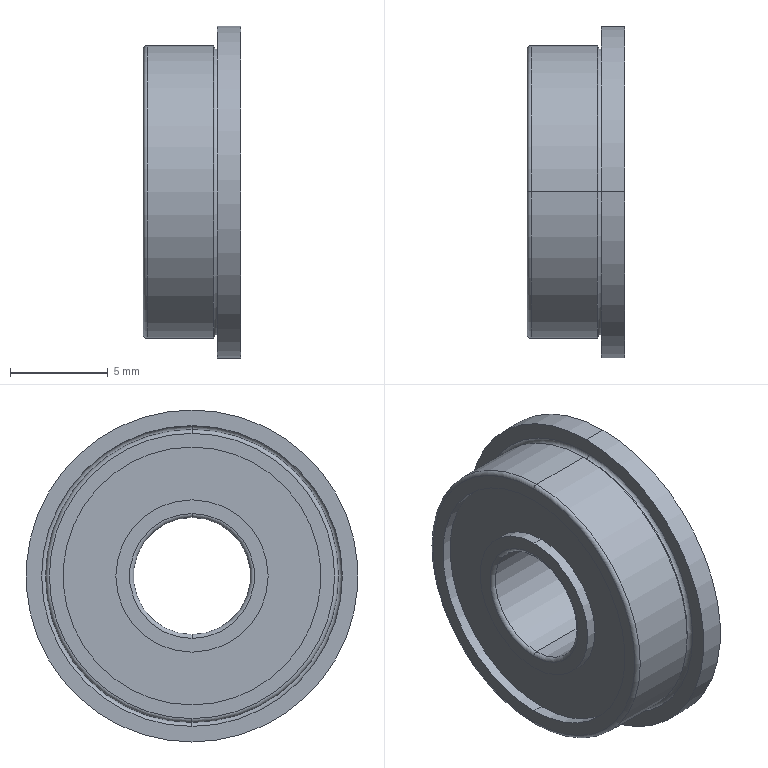Part | SolidWorks | features RefAxis 3, 3DProfileFeature 1, Revolution 1 | 1 solid | 31 faces | box 5 x 17 x 17 mm | volume 704.07 mm3 | cylinder 14 | torus 10 | plane 7 | commonest cylinder face diameters 7.8 x4 13.2 x4 6 x2 15 x2 17 x2
STEP:
#1=CARTESIAN_POINT('',(3.6,0.,7.5));
#2=VERTEX_POINT('',#1);
#3=CARTESIAN_POINT('',(3.8,0.,7.3));
#4=VERTEX_POINT('',#3);
#5=CARTESIAN_POINT('',(3.8,0.,7.5));
#6=DIRECTION('',(0.,-1.,0.));
#7=DIRECTION('',(0.,0.,-1.));
#8=AXIS2_PLACEMENT_3D('',#5,#6,#7);
#9=CIRCLE('',#8,0.2);
#10=EDGE_CURVE('',#2,#4,#9,.T.);
#11=ORIENTED_EDGE('',*,*,#10,.T.);
#12=CARTESIAN_POINT('',(3.8,0.,-7.3));
#13=VERTEX_POINT('',#12);
#14=CARTESIAN_POINT('',(3.8,0.,0.));
#15=DIRECTION('',(-1.,0.,0.));
#16=DIRECTION('',(0.,0.,1.));
#17=AXIS2_PLACEMENT_3D('',#14,#15,#16);
#18=CIRCLE('',#17,7.3);
#19=EDGE_CURVE('',#4,#13,#18,.T.);
#20=ORIENTED_EDGE('',*,*,#19,.T.);
#21=CARTESIAN_POINT('',(3.6,0.,-7.5));
#22=VERTEX_POINT('',#21);
#23=CARTESIAN_POINT('',(3.8,0.,-7.5));
#24=DIRECTION('',(0.,1.,0.));
#25=DIRECTION('',(0.,0.,1.));
#26=AXIS2_PLACEMENT_3D('',#23,#24,#25);
#27=CIRCLE('',#26,0.2);
#28=EDGE_CURVE('',#22,#13,#27,.T.);
#29=ORIENTED_EDGE('',*,*,#28,.F.);
#30=CARTESIAN_POINT('',(3.6,0.,0.));
#31=DIRECTION('',(-1.,0.,0.));
#32=DIRECTION('',(0.,0.,1.));
#33=AXIS2_PLACEMENT_3D('',#30,#31,#32);
#34=CIRCLE('',#33,7.5);
#35=EDGE_CURVE('',#2,#22,#34,.T.);
#36=ORIENTED_EDGE('',*,*,#35,.F.);
#37=EDGE_LOOP('',(#11,#20,#29,#36));
#38=FACE_OUTER_BOUND('',#37,.T.);
#39=CARTESIAN_POINT('',(3.8,0.,0.));
#40=DIRECTION('',(-1.,0.,0.));
#41=DIRECTION('',(0.,0.,1.));
#42=AXIS2_PLACEMENT_3D('',#39,#40,#41);
#43=TOROIDAL_SURFACE('',#42,7.5,0.2);
#44=ADVANCED_FACE('',(#38),#43,.F.);
#45=ORIENTED_EDGE('',*,*,#28,.T.);
#46=CARTESIAN_POINT('',(3.8,0.,0.));
#47=DIRECTION('',(-1.,0.,0.));
#48=DIRECTION('',(0.,0.,1.));
#49=AXIS2_PLACEMENT_3D('',#46,#47,#48);
#50=CIRCLE('',#49,7.3);
#51=EDGE_CURVE('',#13,#4,#50,.T.);
#52=ORIENTED_EDGE('',*,*,#51,.T.);
#53=ORIENTED_EDGE('',*,*,#10,.F.);
#54=CARTESIAN_POINT('',(3.6,0.,0.));
#55=DIRECTION('',(-1.,0.,0.));
#56=DIRECTION('',(0.,0.,1.));
#57=AXIS2_PLACEMENT_3D('',#54,#55,#56);
#58=CIRCLE('',#57,7.5);
#59=EDGE_CURVE('',#22,#2,#58,.T.);
#60=ORIENTED_EDGE('',*,*,#59,.F.);
#61=EDGE_LOOP('',(#45,#52,#53,#60));
#62=FACE_OUTER_BOUND('',#61,.T.);
#63=CARTESIAN_POINT('',(3.8,0.,0.));
#64=DIRECTION('',(-1.,0.,0.));
#65=DIRECTION('',(0.,0.,1.));
#66=AXIS2_PLACEMENT_3D('',#63,#64,#65);
#67=TOROIDAL_SURFACE('',#66,7.5,0.2);
#68=ADVANCED_FACE('',(#62),#67,.F.);
#69=ORIENTED_EDGE('',*,*,#35,.T.);
#70=CARTESIAN_POINT('',(0.2,0.,-7.5));
#71=VERTEX_POINT('',#70);
#72=CARTESIAN_POINT('',(15.,0.,-7.5));
#73=DIRECTION('',(-1.,0.,0.));
#74=VECTOR('',#73,1000.);
#75=LINE('',#72,#74);
#76=EDGE_CURVE('',#22,#71,#75,.T.);
#77=ORIENTED_EDGE('',*,*,#76,.T.);
#78=CARTESIAN_POINT('',(0.2,0.,7.5));
#79=VERTEX_POINT('',#78);
#80=CARTESIAN_POINT('',(0.2,0.,0.));
#81=DIRECTION('',(-1.,0.,0.));
#82=DIRECTION('',(0.,0.,1.));
#83=AXIS2_PLACEMENT_3D('',#80,#81,#82);
#84=CIRCLE('',#83,7.5);
#85=EDGE_CURVE('',#79,#71,#84,.T.);
#86=ORIENTED_EDGE('',*,*,#85,.F.);
#87=CARTESIAN_POINT('',(15.,0.,7.5));
#88=DIRECTION('',(-1.,0.,0.));
#89=VECTOR('',#88,1000.);
#90=LINE('',#87,#89);
#91=EDGE_CURVE('',#2,#79,#90,.T.);
#92=ORIENTED_EDGE('',*,*,#91,.F.);
#93=EDGE_LOOP('',(#69,#77,#86,#92));
#94=FACE_OUTER_BOUND('',#93,.T.);
#95=CARTESIAN_POINT('',(15.,0.,0.));
#96=DIRECTION('',(-1.,0.,0.));
#97=DIRECTION('',(0.,0.,1.));
#98=AXIS2_PLACEMENT_3D('',#95,#96,#97);
#99=CYLINDRICAL_SURFACE('',#98,7.5);
#100=ADVANCED_FACE('',(#94),#99,.T.);
#101=ORIENTED_EDGE('',*,*,#51,.F.);
#102=CARTESIAN_POINT('',(3.8,0.,-7.7));
#103=VERTEX_POINT('',#102);
#104=CARTESIAN_POINT('',(3.8,0.,-7.5));
#105=DIRECTION('',(0.,1.,0.));
#106=DIRECTION('',(0.,0.,1.));
#107=AXIS2_PLACEMENT_3D('',#104,#105,#106);
#108=CIRCLE('',#107,0.2);
#109=EDGE_CURVE('',#13,#103,#108,.T.);
#110=ORIENTED_EDGE('',*,*,#109,.T.);
#111=CARTESIAN_POINT('',(3.8,0.,7.7));
#112=VERTEX_POINT('',#111);
#113=CARTESIAN_POINT('',(3.8,0.,0.));
#114=DIRECTION('',(-1.,0.,0.));
#115=DIRECTION('',(0.,0.,1.));
#116=AXIS2_PLACEMENT_3D('',#113,#114,#115);
#117=CIRCLE('',#116,7.7);
#118=EDGE_CURVE('',#103,#112,#117,.T.);
#119=ORIENTED_EDGE('',*,*,#118,.T.);
#120=CARTESIAN_POINT('',(3.8,0.,7.5));
#121=DIRECTION('',(0.,-1.,0.));
#122=DIRECTION('',(0.,0.,-1.));
#123=AXIS2_PLACEMENT_3D('',#120,#121,#122);
#124=CIRCLE('',#123,0.2);
#125=EDGE_CURVE('',#4,#112,#124,.T.);
#126=ORIENTED_EDGE('',*,*,#125,.F.);
#127=EDGE_LOOP('',(#101,#110,#119,#126));
#128=FACE_OUTER_BOUND('',#127,.T.);
#129=CARTESIAN_POINT('',(3.8,0.,0.));
#130=DIRECTION('',(-1.,0.,0.));
#131=DIRECTION('',(0.,0.,1.));
#132=AXIS2_PLACEMENT_3D('',#129,#130,#131);
#133=TOROIDAL_SURFACE('',#132,7.5,0.2);
#134=ADVANCED_FACE('',(#128),#133,.F.);
#135=CARTESIAN_POINT('',(5.,0.,8.5));
#136=VERTEX_POINT('',#135);
#137=CARTESIAN_POINT('',(5.,0.,-8.5));
#138=VERTEX_POINT('',#137);
#139=CARTESIAN_POINT('',(5.,0.,0.));
#140=DIRECTION('',(-1.,0.,0.));
#141=DIRECTION('',(0.,0.,1.));
#142=AXIS2_PLACEMENT_3D('',#139,#140,#141);
#143=CIRCLE('',#142,8.5);
#144=EDGE_CURVE('',#136,#138,#143,.T.);
#145=ORIENTED_EDGE('',*,*,#144,.T.);
#146=CARTESIAN_POINT('',(3.8,0.,-8.5));
#147=VERTEX_POINT('',#146);
#148=CARTESIAN_POINT('',(15.,0.,-8.5));
#149=DIRECTION('',(-1.,0.,0.));
#150=VECTOR('',#149,1000.);
#151=LINE('',#148,#150);
#152=EDGE_CURVE('',#138,#147,#151,.T.);
#153=ORIENTED_EDGE('',*,*,#152,.T.);
#154=CARTESIAN_POINT('',(3.8,0.,8.5));
#155=VERTEX_POINT('',#154);
#156=CARTESIAN_POINT('',(3.8,0.,0.));
#157=DIRECTION('',(-1.,0.,0.));
#158=DIRECTION('',(0.,0.,1.));
#159=AXIS2_PLACEMENT_3D('',#156,#157,#158);
#160=CIRCLE('',#159,8.5);
#161=EDGE_CURVE('',#155,#147,#160,.T.);
#162=ORIENTED_EDGE('',*,*,#161,.F.);
#163=CARTESIAN_POINT('',(15.,0.,8.5));
#164=DIRECTION('',(-1.,0.,0.));
#165=VECTOR('',#164,1000.);
#166=LINE('',#163,#165);
#167=EDGE_CURVE('',#136,#155,#166,.T.);
#168=ORIENTED_EDGE('',*,*,#167,.F.);
#169=EDGE_LOOP('',(#145,#153,#162,#168));
#170=FACE_OUTER_BOUND('',#169,.T.);
#171=CARTESIAN_POINT('',(15.,0.,0.));
#172=DIRECTION('',(-1.,0.,0.));
#173=DIRECTION('',(0.,0.,1.));
#174=AXIS2_PLACEMENT_3D('',#171,#172,#173);
#175=CYLINDRICAL_SURFACE('',#174,8.5);
#176=ADVANCED_FACE('',(#170),#175,.T.);
#177=CARTESIAN_POINT('',(5.,0.,-6.6));
#178=VERTEX_POINT('',#177);
#179=CARTESIAN_POINT('',(5.,0.,6.6));
#180=VERTEX_POINT('',#179);
#181=CARTESIAN_POINT('',(5.,0.,0.));
#182=DIRECTION('',(-1.,0.,0.));
#183=DIRECTION('',(0.,0.,1.));
#184=AXIS2_PLACEMENT_3D('',#181,#182,#183);
#185=CIRCLE('',#184,6.6);
#186=EDGE_CURVE('',#178,#180,#185,.T.);
#187=ORIENTED_EDGE('',*,*,#186,.F.);
#188=CARTESIAN_POINT('',(4.476,0.,-6.6));
#189=VERTEX_POINT('',#188);
#190=CARTESIAN_POINT('',(15.,0.,-6.6));
#191=DIRECTION('',(-1.,0.,0.));
#192=VECTOR('',#191,1000.);
#193=LINE('',#190,#192);
#194=EDGE_CURVE('',#178,#189,#193,.T.);
#195=ORIENTED_EDGE('',*,*,#194,.T.);
#196=CARTESIAN_POINT('',(4.476,0.,6.6));
#197=VERTEX_POINT('',#196);
#198=CARTESIAN_POINT('',(4.476,0.,0.));
#199=DIRECTION('',(-1.,0.,0.));
#200=DIRECTION('',(0.,0.,1.));
#201=AXIS2_PLACEMENT_3D('',#198,#199,#200);
#202=CIRCLE('',#201,6.6);
#203=EDGE_CURVE('',#189,#197,#202,.T.);
#204=ORIENTED_EDGE('',*,*,#203,.T.);
#205=CARTESIAN_POINT('',(15.,0.,6.6));
#206=DIRECTION('',(-1.,0.,0.));
#207=VECTOR('',#206,1000.);
#208=LINE('',#205,#207);
#209=EDGE_CURVE('',#180,#197,#208,.T.);
#210=ORIENTED_EDGE('',*,*,#209,.F.);
#211=EDGE_LOOP('',(#187,#195,#204,#210));
#212=FACE_OUTER_BOUND('',#211,.T.);
#213=CARTESIAN_POINT('',(15.,0.,0.));
#214=DIRECTION('',(-1.,0.,0.));
#215=DIRECTION('',(0.,0.,1.));
#216=AXIS2_PLACEMENT_3D('',#213,#214,#215);
#217=CYLINDRICAL_SURFACE('',#216,6.6);
#218=ADVANCED_FACE('',(#212),#217,.F.);
#219=CARTESIAN_POINT('',(5.,0.,3.9));
#220=VERTEX_POINT('',#219);
#221=CARTESIAN_POINT('',(5.,0.,-3.9));
#222=VERTEX_POINT('',#221);
#223=CARTESIAN_POINT('',(5.,0.,0.));
#224=DIRECTION('',(-1.,0.,0.));
#225=DIRECTION('',(0.,0.,1.));
#226=AXIS2_PLACEMENT_3D('',#223,#224,#225);
#227=CIRCLE('',#226,3.9);
#228=EDGE_CURVE('',#220,#222,#227,.T.);
#229=ORIENTED_EDGE('',*,*,#228,.T.);
#230=CARTESIAN_POINT('',(4.476,0.,-3.9));
#231=VERTEX_POINT('',#230);
#232=CARTESIAN_POINT('',(15.,0.,-3.9));
#233=DIRECTION('',(-1.,0.,0.));
#234=VECTOR('',#233,1000.);
#235=LINE('',#232,#234);
#236=EDGE_CURVE('',#222,#231,#235,.T.);
#237=ORIENTED_EDGE('',*,*,#236,.T.);
#238=CARTESIAN_POINT('',(4.476,0.,3.9));
#239=VERTEX_POINT('',#238);
#240=CARTESIAN_POINT('',(4.476,0.,0.));
#241=DIRECTION('',(-1.,0.,0.));
#242=DIRECTION('',(0.,0.,1.));
#243=AXIS2_PLACEMENT_3D('',#240,#241,#242);
#244=CIRCLE('',#243,3.9);
#245=EDGE_CURVE('',#239,#231,#244,.T.);
#246=ORIENTED_EDGE('',*,*,#245,.F.);
#247=CARTESIAN_POINT('',(15.,0.,3.9));
#248=DIRECTION('',(-1.,0.,0.));
#249=VECTOR('',#248,1000.);
#250=LINE('',#247,#249);
#251=EDGE_CURVE('',#220,#239,#250,.T.);
#252=ORIENTED_EDGE('',*,*,#251,.F.);
#253=EDGE_LOOP('',(#229,#237,#246,#252));
#254=FACE_OUTER_BOUND('',#253,.T.);
#255=CARTESIAN_POINT('',(15.,0.,0.));
#256=DIRECTION('',(-1.,0.,0.));
#257=DIRECTION('',(0.,0.,1.));
#258=AXIS2_PLACEMENT_3D('',#255,#256,#257);
#259=CYLINDRICAL_SURFACE('',#258,3.9);
#260=ADVANCED_FACE('',(#254),#259,.T.);
#261=CARTESIAN_POINT('',(4.8,0.,3.));
#262=VERTEX_POINT('',#261);
#263=CARTESIAN_POINT('',(4.8,0.,-3.));
#264=VERTEX_POINT('',#263);
#265=CARTESIAN_POINT('',(4.8,0.,0.));
#266=DIRECTION('',(-1.,0.,0.));
#267=DIRECTION('',(0.,0.,1.));
#268=AXIS2_PLACEMENT_3D('',#265,#266,#267);
#269=CIRCLE('',#268,3.);
#270=EDGE_CURVE('',#262,#264,#269,.T.);
#271=ORIENTED_EDGE('',*,*,#270,.T.);
#272=CARTESIAN_POINT('',(5.,0.,-3.2));
#273=VERTEX_POINT('',#272);
#274=CARTESIAN_POINT('',(4.8,0.,-3.2));
#275=DIRECTION('',(0.,1.,0.));
#276=DIRECTION('',(0.,0.,1.));
#277=AXIS2_PLACEMENT_3D('',#274,#275,#276);
#278=CIRCLE('',#277,0.2);
#279=EDGE_CURVE('',#264,#273,#278,.T.);
#280=ORIENTED_EDGE('',*,*,#279,.T.);
#281=CARTESIAN_POINT('',(5.,0.,3.2));
#282=VERTEX_POINT('',#281);
#283=CARTESIAN_POINT('',(5.,0.,0.));
#284=DIRECTION('',(-1.,0.,0.));
#285=DIRECTION('',(0.,0.,1.));
#286=AXIS2_PLACEMENT_3D('',#283,#284,#285);
#287=CIRCLE('',#286,3.2);
#288=EDGE_CURVE('',#282,#273,#287,.T.);
#289=ORIENTED_EDGE('',*,*,#288,.F.);
#290=CARTESIAN_POINT('',(4.8,0.,3.2));
#291=DIRECTION('',(0.,-1.,0.));
#292=DIRECTION('',(0.,0.,-1.));
#293=AXIS2_PLACEMENT_3D('',#290,#291,#292);
#294=CIRCLE('',#293,0.2);
#295=EDGE_CURVE('',#262,#282,#294,.T.);
#296=ORIENTED_EDGE('',*,*,#295,.F.);
#297=EDGE_LOOP('',(#271,#280,#289,#296));
#298=FACE_OUTER_BOUND('',#297,.T.);
#299=CARTESIAN_POINT('',(4.8,0.,0.));
#300=DIRECTION('',(-1.,0.,0.));
#301=DIRECTION('',(0.,0.,1.));
#302=AXIS2_PLACEMENT_3D('',#299,#300,#301);
#303=TOROIDAL_SURFACE('',#302,3.2,0.2);
#304=ADVANCED_FACE('',(#298),#303,.T.);
#305=CARTESIAN_POINT('',(4.8,0.,0.));
#306=DIRECTION('',(-1.,0.,0.));
#307=DIRECTION('',(0.,0.,1.));
#308=AXIS2_PLACEMENT_3D('',#305,#306,#307);
#309=CIRCLE('',#308,3.);
#310=EDGE_CURVE('',#264,#262,#309,.T.);
#311=ORIENTED_EDGE('',*,*,#310,.F.);
#312=CARTESIAN_POINT('',(0.2,0.,-3.));
#313=VERTEX_POINT('',#312);
#314=CARTESIAN_POINT('',(15.,0.,-3.));
#315=DIRECTION('',(-1.,0.,0.));
#316=VECTOR('',#315,1000.);
#317=LINE('',#314,#316);
#318=EDGE_CURVE('',#264,#313,#317,.T.);
#319=ORIENTED_EDGE('',*,*,#318,.T.);
#320=CARTESIAN_POINT('',(0.2,0.,3.));
#321=VERTEX_POINT('',#320);
#322=CARTESIAN_POINT('',(0.2,0.,0.));
#323=DIRECTION('',(-1.,0.,0.));
#324=DIRECTION('',(0.,0.,1.));
#325=AXIS2_PLACEMENT_3D('',#322,#323,#324);
#326=CIRCLE('',#325,3.);
#327=EDGE_CURVE('',#313,#321,#326,.T.);
#328=ORIENTED_EDGE('',*,*,#327,.T.);
#329=CARTESIAN_POINT('',(15.,0.,3.));
#330=DIRECTION('',(-1.,0.,0.));
#331=VECTOR('',#330,1000.);
#332=LINE('',#329,#331);
#333=EDGE_CURVE('',#262,#321,#332,.T.);
#334=ORIENTED_EDGE('',*,*,#333,.F.);
#335=EDGE_LOOP('',(#311,#319,#328,#334));
#336=FACE_OUTER_BOUND('',#335,.T.);
#337=CARTESIAN_POINT('',(15.,0.,0.));
#338=DIRECTION('',(-1.,0.,0.));
#339=DIRECTION('',(0.,0.,1.));
#340=AXIS2_PLACEMENT_3D('',#337,#338,#339);
#341=CYLINDRICAL_SURFACE('',#340,3.);
#342=ADVANCED_FACE('',(#336),#341,.F.);
#343=CARTESIAN_POINT('',(0.,0.,3.2));
#344=VERTEX_POINT('',#343);
#345=CARTESIAN_POINT('',(0.,0.,-3.2));
#346=VERTEX_POINT('',#345);
#347=CARTESIAN_POINT('',(0.,0.,0.));
#348=DIRECTION('',(-1.,0.,0.));
#349=DIRECTION('',(0.,0.,1.));
#350=AXIS2_PLACEMENT_3D('',#347,#348,#349);
#351=CIRCLE('',#350,3.2);
#352=EDGE_CURVE('',#344,#346,#351,.T.);
#353=ORIENTED_EDGE('',*,*,#352,.T.);
#354=CARTESIAN_POINT('',(0.2,0.,-3.2));
#355=DIRECTION('',(0.,1.,0.));
#356=DIRECTION('',(0.,0.,1.));
#357=AXIS2_PLACEMENT_3D('',#354,#355,#356);
#358=CIRCLE('',#357,0.2);
#359=EDGE_CURVE('',#346,#313,#358,.T.);
#360=ORIENTED_EDGE('',*,*,#359,.T.);
#361=CARTESIAN_POINT('',(0.2,0.,0.));
#362=DIRECTION('',(-1.,0.,0.));
#363=DIRECTION('',(0.,0.,1.));
#364=AXIS2_PLACEMENT_3D('',#361,#362,#363);
#365=CIRCLE('',#364,3.);
#366=EDGE_CURVE('',#321,#313,#365,.T.);
#367=ORIENTED_EDGE('',*,*,#366,.F.);
#368=CARTESIAN_POINT('',(0.2,0.,3.2));
#369=DIRECTION('',(0.,-1.,0.));
#370=DIRECTION('',(0.,0.,-1.));
#371=AXIS2_PLACEMENT_3D('',#368,#369,#370);
#372=CIRCLE('',#371,0.2);
#373=EDGE_CURVE('',#344,#321,#372,.T.);
#374=ORIENTED_EDGE('',*,*,#373,.F.);
#375=EDGE_LOOP('',(#353,#360,#367,#374));
#376=FACE_OUTER_BOUND('',#375,.T.);
#377=CARTESIAN_POINT('',(0.2,0.,0.));
#378=DIRECTION('',(-1.,0.,0.));
#379=DIRECTION('',(0.,0.,1.));
#380=AXIS2_PLACEMENT_3D('',#377,#378,#379);
#381=TOROIDAL_SURFACE('',#380,3.2,0.2);
#382=ADVANCED_FACE('',(#376),#381,.T.);
#383=CARTESIAN_POINT('',(0.5237,0.,3.9));
#384=VERTEX_POINT('',#383);
#385=CARTESIAN_POINT('',(0.5237,0.,-3.9));
#386=VERTEX_POINT('',#385);
#387=CARTESIAN_POINT('',(0.5237,0.,0.));
#388=DIRECTION('',(-1.,0.,0.));
#389=DIRECTION('',(0.,0.,1.));
#390=AXIS2_PLACEMENT_3D('',#387,#388,#389);
#391=CIRCLE('',#390,3.9);
#392=EDGE_CURVE('',#384,#386,#391,.T.);
#393=ORIENTED_EDGE('',*,*,#392,.T.);
#394=CARTESIAN_POINT('',(0.,0.,-3.9));
#395=VERTEX_POINT('',#394);
#396=CARTESIAN_POINT('',(15.,0.,-3.9));
#397=DIRECTION('',(-1.,0.,0.));
#398=VECTOR('',#397,1000.);
#399=LINE('',#396,#398);
#400=EDGE_CURVE('',#386,#395,#399,.T.);
#401=ORIENTED_EDGE('',*,*,#400,.T.);
#402=CARTESIAN_POINT('',(0.,0.,3.9));
#403=VERTEX_POINT('',#402);
#404=CARTESIAN_POINT('',(0.,0.,0.));
#405=DIRECTION('',(-1.,0.,0.));
#406=DIRECTION('',(0.,0.,1.));
#407=AXIS2_PLACEMENT_3D('',#404,#405,#406);
#408=CIRCLE('',#407,3.9);
#409=EDGE_CURVE('',#403,#395,#408,.T.);
#410=ORIENTED_EDGE('',*,*,#409,.F.);
#411=CARTESIAN_POINT('',(15.,0.,3.9));
#412=DIRECTION('',(-1.,0.,0.));
#413=VECTOR('',#412,1000.);
#414=LINE('',#411,#413);
#415=EDGE_CURVE('',#384,#403,#414,.T.);
#416=ORIENTED_EDGE('',*,*,#415,.F.);
#417=EDGE_LOOP('',(#393,#401,#410,#416));
#418=FACE_OUTER_BOUND('',#417,.T.);
#419=CARTESIAN_POINT('',(15.,0.,0.));
#420=DIRECTION('',(-1.,0.,0.));
#421=DIRECTION('',(0.,0.,1.));
#422=AXIS2_PLACEMENT_3D('',#419,#420,#421);
#423=CYLINDRICAL_SURFACE('',#422,3.9);
#424=ADVANCED_FACE('',(#418),#423,.T.);
#425=CARTESIAN_POINT('',(0.5237,0.,-6.6));
#426=VERTEX_POINT('',#425);
#427=CARTESIAN_POINT('',(0.5237,0.,6.6));
#428=VERTEX_POINT('',#427);
#429=CARTESIAN_POINT('',(0.5237,0.,0.));
#430=DIRECTION('',(-1.,0.,0.));
#431=DIRECTION('',(0.,0.,1.));
#432=AXIS2_PLACEMENT_3D('',#429,#430,#431);
#433=CIRCLE('',#432,6.6);
#434=EDGE_CURVE('',#426,#428,#433,.T.);
#435=ORIENTED_EDGE('',*,*,#434,.F.);
#436=CARTESIAN_POINT('',(0.,0.,-6.6));
#437=VERTEX_POINT('',#436);
#438=CARTESIAN_POINT('',(15.,0.,-6.6));
#439=DIRECTION('',(-1.,0.,0.));
#440=VECTOR('',#439,1000.);
#441=LINE('',#438,#440);
#442=EDGE_CURVE('',#426,#437,#441,.T.);
#443=ORIENTED_EDGE('',*,*,#442,.T.);
#444=CARTESIAN_POINT('',(0.,0.,6.6));
#445=VERTEX_POINT('',#444);
#446=CARTESIAN_POINT('',(0.,0.,0.));
#447=DIRECTION('',(-1.,0.,0.));
#448=DIRECTION('',(0.,0.,1.));
#449=AXIS2_PLACEMENT_3D('',#446,#447,#448);
#450=CIRCLE('',#449,6.6);
#451=EDGE_CURVE('',#437,#445,#450,.T.);
#452=ORIENTED_EDGE('',*,*,#451,.T.);
#453=CARTESIAN_POINT('',(15.,0.,6.6));
#454=DIRECTION('',(-1.,0.,0.));
#455=VECTOR('',#454,1000.);
#456=LINE('',#453,#455);
#457=EDGE_CURVE('',#428,#445,#456,.T.);
#458=ORIENTED_EDGE('',*,*,#457,.F.);
#459=EDGE_LOOP('',(#435,#443,#452,#458));
#460=FACE_OUTER_BOUND('',#459,.T.);
#461=CARTESIAN_POINT('',(15.,0.,0.));
#462=DIRECTION('',(-1.,0.,0.));
#463=DIRECTION('',(0.,0.,1.));
#464=AXIS2_PLACEMENT_3D('',#461,#462,#463);
#465=CYLINDRICAL_SURFACE('',#464,6.6);
#466=ADVANCED_FACE('',(#460),#465,.F.);
#467=ORIENTED_EDGE('',*,*,#85,.T.);
#468=CARTESIAN_POINT('',(0.,0.,-7.3));
#469=VERTEX_POINT('',#468);
#470=CARTESIAN_POINT('',(0.2,0.,-7.3));
#471=DIRECTION('',(0.,1.,0.));
#472=DIRECTION('',(0.,0.,1.));
#473=AXIS2_PLACEMENT_3D('',#470,#471,#472);
#474=CIRCLE('',#473,0.2);
#475=EDGE_CURVE('',#71,#469,#474,.T.);
#476=ORIENTED_EDGE('',*,*,#475,.T.);
#477=CARTESIAN_POINT('',(0.,0.,7.3));
#478=VERTEX_POINT('',#477);
#479=CARTESIAN_POINT('',(0.,0.,0.));
#480=DIRECTION('',(-1.,0.,0.));
#481=DIRECTION('',(0.,0.,1.));
#482=AXIS2_PLACEMENT_3D('',#479,#480,#481);
#483=CIRCLE('',#482,7.3);
#484=EDGE_CURVE('',#478,#469,#483,.T.);
#485=ORIENTED_EDGE('',*,*,#484,.F.);
#486=CARTESIAN_POINT('',(0.2,0.,7.3));
#487=DIRECTION('',(0.,-1.,0.));
#488=DIRECTION('',(0.,0.,-1.));
#489=AXIS2_PLACEMENT_3D('',#486,#487,#488);
#490=CIRCLE('',#489,0.2);
#491=EDGE_CURVE('',#79,#478,#490,.T.);
#492=ORIENTED_EDGE('',*,*,#491,.F.);
#493=EDGE_LOOP('',(#467,#476,#485,#492));
#494=FACE_OUTER_BOUND('',#493,.T.);
#495=CARTESIAN_POINT('',(0.2,0.,0.));
#496=DIRECTION('',(-1.,0.,0.));
#497=DIRECTION('',(0.,0.,1.));
#498=AXIS2_PLACEMENT_3D('',#495,#496,#497);
#499=TOROIDAL_SURFACE('',#498,7.3,0.2);
#500=ADVANCED_FACE('',(#494),#499,.T.);
#501=ORIENTED_EDGE('',*,*,#475,.F.);
#502=CARTESIAN_POINT('',(0.2,0.,0.));
#503=DIRECTION('',(-1.,0.,0.));
#504=DIRECTION('',(0.,0.,1.));
#505=AXIS2_PLACEMENT_3D('',#502,#503,#504);
#506=CIRCLE('',#505,7.5);
#507=EDGE_CURVE('',#71,#79,#506,.T.);
#508=ORIENTED_EDGE('',*,*,#507,.T.);
#509=ORIENTED_EDGE('',*,*,#491,.T.);
#510=CARTESIAN_POINT('',(0.,0.,0.));
#511=DIRECTION('',(-1.,0.,0.));
#512=DIRECTION('',(0.,0.,1.));
#513=AXIS2_PLACEMENT_3D('',#510,#511,#512);
#514=CIRCLE('',#513,7.3);
#515=EDGE_CURVE('',#469,#478,#514,.T.);
#516=ORIENTED_EDGE('',*,*,#515,.F.);
#517=EDGE_LOOP('',(#501,#508,#509,#516));
#518=FACE_OUTER_BOUND('',#517,.T.);
#519=CARTESIAN_POINT('',(0.2,0.,0.));
#520=DIRECTION('',(-1.,0.,0.));
#521=DIRECTION('',(0.,0.,1.));
#522=AXIS2_PLACEMENT_3D('',#519,#520,#521);
#523=TOROIDAL_SURFACE('',#522,7.3,0.2);
#524=ADVANCED_FACE('',(#518),#523,.T.);
#525=CARTESIAN_POINT('',(0.,0.,0.));
#526=DIRECTION('',(-1.,0.,0.));
#527=DIRECTION('',(0.,0.,1.));
#528=AXIS2_PLACEMENT_3D('',#525,#526,#527);
#529=CIRCLE('',#528,6.6);
#530=EDGE_CURVE('',#445,#437,#529,.T.);
#531=ORIENTED_EDGE('',*,*,#530,.F.);
#532=ORIENTED_EDGE('',*,*,#451,.F.);
#533=EDGE_LOOP('',(#531,#532));
#534=FACE_BOUND('',#533,.T.);
#535=ORIENTED_EDGE('',*,*,#484,.T.);
#536=ORIENTED_EDGE('',*,*,#515,.T.);
#537=EDGE_LOOP('',(#535,#536));
#538=FACE_OUTER_BOUND('',#537,.T.);
#539=CARTESIAN_POINT('',(0.,7.3,0.));
#540=DIRECTION('',(1.,0.,0.));
#541=DIRECTION('',(0.,0.,-1.));
#542=AXIS2_PLACEMENT_3D('',#539,#540,#541);
#543=PLANE('',#542);
#544=ADVANCED_FACE('',(#534,#538),#543,.F.);
#545=ORIENTED_EDGE('',*,*,#442,.F.);
#546=CARTESIAN_POINT('',(0.5237,0.,0.));
#547=DIRECTION('',(-1.,0.,0.));
#548=DIRECTION('',(0.,0.,1.));
#549=AXIS2_PLACEMENT_3D('',#546,#547,#548);
#550=CIRCLE('',#549,6.6);
#551=EDGE_CURVE('',#428,#426,#550,.T.);
#552=ORIENTED_EDGE('',*,*,#551,.F.);
#553=ORIENTED_EDGE('',*,*,#457,.T.);
#554=ORIENTED_EDGE('',*,*,#530,.T.);
#555=EDGE_LOOP('',(#545,#552,#553,#554));
#556=FACE_OUTER_BOUND('',#555,.T.);
#557=CARTESIAN_POINT('',(15.,0.,0.));
#558=DIRECTION('',(-1.,0.,0.));
#559=DIRECTION('',(0.,0.,1.));
#560=AXIS2_PLACEMENT_3D('',#557,#558,#559);
#561=CYLINDRICAL_SURFACE('',#560,6.6);
#562=ADVANCED_FACE('',(#556),#561,.F.);
#563=ORIENTED_EDGE('',*,*,#392,.F.);
#564=CARTESIAN_POINT('',(0.5237,0.,0.));
#565=DIRECTION('',(-1.,0.,0.));
#566=DIRECTION('',(0.,0.,1.));
#567=AXIS2_PLACEMENT_3D('',#564,#565,#566);
#568=CIRCLE('',#567,3.9);
#569=EDGE_CURVE('',#386,#384,#568,.T.);
#570=ORIENTED_EDGE('',*,*,#569,.F.);
#571=EDGE_LOOP('',(#563,#570));
#572=FACE_BOUND('',#571,.T.);
#573=ORIENTED_EDGE('',*,*,#551,.T.);
#574=ORIENTED_EDGE('',*,*,#434,.T.);
#575=EDGE_LOOP('',(#573,#574));
#576=FACE_OUTER_BOUND('',#575,.T.);
#577=CARTESIAN_POINT('',(0.5237,6.6,0.));
#578=DIRECTION('',(1.,0.,0.));
#579=DIRECTION('',(0.,0.,-1.));
#580=AXIS2_PLACEMENT_3D('',#577,#578,#579);
#581=PLANE('',#580);
#582=ADVANCED_FACE('',(#572,#576),#581,.F.);
#583=ORIENTED_EDGE('',*,*,#400,.F.);
#584=ORIENTED_EDGE('',*,*,#569,.T.);
#585=ORIENTED_EDGE('',*,*,#415,.T.);
#586=CARTESIAN_POINT('',(0.,0.,0.));
#587=DIRECTION('',(-1.,0.,0.));
#588=DIRECTION('',(0.,0.,1.));
#589=AXIS2_PLACEMENT_3D('',#586,#587,#588);
#590=CIRCLE('',#589,3.9);
#591=EDGE_CURVE('',#395,#403,#590,.T.);
#592=ORIENTED_EDGE('',*,*,#591,.F.);
#593=EDGE_LOOP('',(#583,#584,#585,#592));
#594=FACE_OUTER_BOUND('',#593,.T.);
#595=CARTESIAN_POINT('',(15.,0.,0.));
#596=DIRECTION('',(-1.,0.,0.));
#597=DIRECTION('',(0.,0.,1.));
#598=AXIS2_PLACEMENT_3D('',#595,#596,#597);
#599=CYLINDRICAL_SURFACE('',#598,3.9);
#600=ADVANCED_FACE('',(#594),#599,.T.);
#601=ORIENTED_EDGE('',*,*,#352,.F.);
#602=CARTESIAN_POINT('',(0.,0.,0.));
#603=DIRECTION('',(-1.,0.,0.));
#604=DIRECTION('',(0.,0.,1.));
#605=AXIS2_PLACEMENT_3D('',#602,#603,#604);
#606=CIRCLE('',#605,3.2);
#607=EDGE_CURVE('',#346,#344,#606,.T.);
#608=ORIENTED_EDGE('',*,*,#607,.F.);
#609=EDGE_LOOP('',(#601,#608));
#610=FACE_BOUND('',#609,.T.);
#611=ORIENTED_EDGE('',*,*,#409,.T.);
#612=ORIENTED_EDGE('',*,*,#591,.T.);
#613=EDGE_LOOP('',(#611,#612));
#614=FACE_OUTER_BOUND('',#613,.T.);
#615=CARTESIAN_POINT('',(0.,3.9,0.));
#616=DIRECTION('',(1.,0.,0.));
#617=DIRECTION('',(0.,0.,-1.));
#618=AXIS2_PLACEMENT_3D('',#615,#616,#617);
#619=PLANE('',#618);
#620=ADVANCED_FACE('',(#610,#614),#619,.F.);
#621=ORIENTED_EDGE('',*,*,#359,.F.);
#622=ORIENTED_EDGE('',*,*,#607,.T.);
#623=ORIENTED_EDGE('',*,*,#373,.T.);
#624=ORIENTED_EDGE('',*,*,#327,.F.);
#625=EDGE_LOOP('',(#621,#622,#623,#624));
#626=FACE_OUTER_BOUND('',#625,.T.);
#627=CARTESIAN_POINT('',(0.2,0.,0.));
#628=DIRECTION('',(-1.,0.,0.));
#629=DIRECTION('',(0.,0.,1.));
#630=AXIS2_PLACEMENT_3D('',#627,#628,#629);
#631=TOROIDAL_SURFACE('',#630,3.2,0.2);
#632=ADVANCED_FACE('',(#626),#631,.T.);
#633=ORIENTED_EDGE('',*,*,#318,.F.);
#634=ORIENTED_EDGE('',*,*,#270,.F.);
#635=ORIENTED_EDGE('',*,*,#333,.T.);
#636=ORIENTED_EDGE('',*,*,#366,.T.);
#637=EDGE_LOOP('',(#633,#634,#635,#636));
#638=FACE_OUTER_BOUND('',#637,.T.);
#639=CARTESIAN_POINT('',(15.,0.,0.));
#640=DIRECTION('',(-1.,0.,0.));
#641=DIRECTION('',(0.,0.,1.));
#642=AXIS2_PLACEMENT_3D('',#639,#640,#641);
#643=CYLINDRICAL_SURFACE('',#642,3.);
#644=ADVANCED_FACE('',(#638),#643,.F.);
#645=ORIENTED_EDGE('',*,*,#279,.F.);
#646=ORIENTED_EDGE('',*,*,#310,.T.);
#647=ORIENTED_EDGE('',*,*,#295,.T.);
#648=CARTESIAN_POINT('',(5.,0.,0.));
#649=DIRECTION('',(-1.,0.,0.));
#650=DIRECTION('',(0.,0.,1.));
#651=AXIS2_PLACEMENT_3D('',#648,#649,#650);
#652=CIRCLE('',#651,3.2);
#653=EDGE_CURVE('',#273,#282,#652,.T.);
#654=ORIENTED_EDGE('',*,*,#653,.F.);
#655=EDGE_LOOP('',(#645,#646,#647,#654));
#656=FACE_OUTER_BOUND('',#655,.T.);
#657=CARTESIAN_POINT('',(4.8,0.,0.));
#658=DIRECTION('',(-1.,0.,0.));
#659=DIRECTION('',(0.,0.,1.));
#660=AXIS2_PLACEMENT_3D('',#657,#658,#659);
#661=TOROIDAL_SURFACE('',#660,3.2,0.2);
#662=ADVANCED_FACE('',(#656),#661,.T.);
#663=ORIENTED_EDGE('',*,*,#228,.F.);
#664=CARTESIAN_POINT('',(5.,0.,0.));
#665=DIRECTION('',(-1.,0.,0.));
#666=DIRECTION('',(0.,0.,1.));
#667=AXIS2_PLACEMENT_3D('',#664,#665,#666);
#668=CIRCLE('',#667,3.9);
#669=EDGE_CURVE('',#222,#220,#668,.T.);
#670=ORIENTED_EDGE('',*,*,#669,.F.);
#671=EDGE_LOOP('',(#663,#670));
#672=FACE_OUTER_BOUND('',#671,.T.);
#673=ORIENTED_EDGE('',*,*,#288,.T.);
#674=ORIENTED_EDGE('',*,*,#653,.T.);
#675=EDGE_LOOP('',(#673,#674));
#676=FACE_BOUND('',#675,.T.);
#677=CARTESIAN_POINT('',(5.,3.2,0.));
#678=DIRECTION('',(-1.,0.,0.));
#679=DIRECTION('',(0.,0.,1.));
#680=AXIS2_PLACEMENT_3D('',#677,#678,#679);
#681=PLANE('',#680);
#682=ADVANCED_FACE('',(#672,#676),#681,.F.);
#683=ORIENTED_EDGE('',*,*,#236,.F.);
#684=ORIENTED_EDGE('',*,*,#669,.T.);
#685=ORIENTED_EDGE('',*,*,#251,.T.);
#686=CARTESIAN_POINT('',(4.476,0.,0.));
#687=DIRECTION('',(-1.,0.,0.));
#688=DIRECTION('',(0.,0.,1.));
#689=AXIS2_PLACEMENT_3D('',#686,#687,#688);
#690=CIRCLE('',#689,3.9);
#691=EDGE_CURVE('',#231,#239,#690,.T.);
#692=ORIENTED_EDGE('',*,*,#691,.F.);
#693=EDGE_LOOP('',(#683,#684,#685,#692));
#694=FACE_OUTER_BOUND('',#693,.T.);
#695=CARTESIAN_POINT('',(15.,0.,0.));
#696=DIRECTION('',(-1.,0.,0.));
#697=DIRECTION('',(0.,0.,1.));
#698=AXIS2_PLACEMENT_3D('',#695,#696,#697);
#699=CYLINDRICAL_SURFACE('',#698,3.9);
#700=ADVANCED_FACE('',(#694),#699,.T.);
#701=CARTESIAN_POINT('',(4.476,0.,0.));
#702=DIRECTION('',(-1.,0.,0.));
#703=DIRECTION('',(0.,0.,1.));
#704=AXIS2_PLACEMENT_3D('',#701,#702,#703);
#705=CIRCLE('',#704,6.6);
#706=EDGE_CURVE('',#197,#189,#705,.T.);
#707=ORIENTED_EDGE('',*,*,#706,.F.);
#708=ORIENTED_EDGE('',*,*,#203,.F.);
#709=EDGE_LOOP('',(#707,#708));
#710=FACE_OUTER_BOUND('',#709,.T.);
#711=ORIENTED_EDGE('',*,*,#245,.T.);
#712=ORIENTED_EDGE('',*,*,#691,.T.);
#713=EDGE_LOOP('',(#711,#712));
#714=FACE_BOUND('',#713,.T.);
#715=CARTESIAN_POINT('',(4.476,3.9,0.));
#716=DIRECTION('',(-1.,0.,0.));
#717=DIRECTION('',(0.,0.,1.));
#718=AXIS2_PLACEMENT_3D('',#715,#716,#717);
#719=PLANE('',#718);
#720=ADVANCED_FACE('',(#710,#714),#719,.F.);
#721=ORIENTED_EDGE('',*,*,#194,.F.);
#722=CARTESIAN_POINT('',(5.,0.,0.));
#723=DIRECTION('',(-1.,0.,0.));
#724=DIRECTION('',(0.,0.,1.));
#725=AXIS2_PLACEMENT_3D('',#722,#723,#724);
#726=CIRCLE('',#725,6.6);
#727=EDGE_CURVE('',#180,#178,#726,.T.);
#728=ORIENTED_EDGE('',*,*,#727,.F.);
#729=ORIENTED_EDGE('',*,*,#209,.T.);
#730=ORIENTED_EDGE('',*,*,#706,.T.);
#731=EDGE_LOOP('',(#721,#728,#729,#730));
#732=FACE_OUTER_BOUND('',#731,.T.);
#733=CARTESIAN_POINT('',(15.,0.,0.));
#734=DIRECTION('',(-1.,0.,0.));
#735=DIRECTION('',(0.,0.,1.));
#736=AXIS2_PLACEMENT_3D('',#733,#734,#735);
#737=CYLINDRICAL_SURFACE('',#736,6.6);
#738=ADVANCED_FACE('',(#732),#737,.F.);
#739=ORIENTED_EDGE('',*,*,#144,.F.);
#740=CARTESIAN_POINT('',(5.,0.,0.));
#741=DIRECTION('',(-1.,0.,0.));
#742=DIRECTION('',(0.,0.,1.));
#743=AXIS2_PLACEMENT_3D('',#740,#741,#742);
#744=CIRCLE('',#743,8.5);
#745=EDGE_CURVE('',#138,#136,#744,.T.);
#746=ORIENTED_EDGE('',*,*,#745,.F.);
#747=EDGE_LOOP('',(#739,#746));
#748=FACE_OUTER_BOUND('',#747,.T.);
#749=ORIENTED_EDGE('',*,*,#727,.T.);
#750=ORIENTED_EDGE('',*,*,#186,.T.);
#751=EDGE_LOOP('',(#749,#750));
#752=FACE_BOUND('',#751,.T.);
#753=CARTESIAN_POINT('',(5.,6.6,0.));
#754=DIRECTION('',(-1.,0.,0.));
#755=DIRECTION('',(0.,0.,1.));
#756=AXIS2_PLACEMENT_3D('',#753,#754,#755);
#757=PLANE('',#756);
#758=ADVANCED_FACE('',(#748,#752),#757,.F.);
#759=ORIENTED_EDGE('',*,*,#152,.F.);
#760=ORIENTED_EDGE('',*,*,#745,.T.);
#761=ORIENTED_EDGE('',*,*,#167,.T.);
#762=CARTESIAN_POINT('',(3.8,0.,0.));
#763=DIRECTION('',(-1.,0.,0.));
#764=DIRECTION('',(0.,0.,1.));
#765=AXIS2_PLACEMENT_3D('',#762,#763,#764);
#766=CIRCLE('',#765,8.5);
#767=EDGE_CURVE('',#147,#155,#766,.T.);
#768=ORIENTED_EDGE('',*,*,#767,.F.);
#769=EDGE_LOOP('',(#759,#760,#761,#768));
#770=FACE_OUTER_BOUND('',#769,.T.);
#771=CARTESIAN_POINT('',(15.,0.,0.));
#772=DIRECTION('',(-1.,0.,0.));
#773=DIRECTION('',(0.,0.,1.));
#774=AXIS2_PLACEMENT_3D('',#771,#772,#773);
#775=CYLINDRICAL_SURFACE('',#774,8.5);
#776=ADVANCED_FACE('',(#770),#775,.T.);
#777=CARTESIAN_POINT('',(3.8,0.,0.));
#778=DIRECTION('',(-1.,0.,0.));
#779=DIRECTION('',(0.,0.,1.));
#780=AXIS2_PLACEMENT_3D('',#777,#778,#779);
#781=CIRCLE('',#780,7.7);
#782=EDGE_CURVE('',#112,#103,#781,.T.);
#783=ORIENTED_EDGE('',*,*,#782,.F.);
#784=ORIENTED_EDGE('',*,*,#118,.F.);
#785=EDGE_LOOP('',(#783,#784));
#786=FACE_BOUND('',#785,.T.);
#787=ORIENTED_EDGE('',*,*,#161,.T.);
#788=ORIENTED_EDGE('',*,*,#767,.T.);
#789=EDGE_LOOP('',(#787,#788));
#790=FACE_OUTER_BOUND('',#789,.T.);
#791=CARTESIAN_POINT('',(3.8,8.5,0.));
#792=DIRECTION('',(1.,0.,0.));
#793=DIRECTION('',(0.,0.,-1.));
#794=AXIS2_PLACEMENT_3D('',#791,#792,#793);
#795=PLANE('',#794);
#796=ADVANCED_FACE('',(#786,#790),#795,.F.);
#797=ORIENTED_EDGE('',*,*,#19,.F.);
#798=ORIENTED_EDGE('',*,*,#125,.T.);
#799=ORIENTED_EDGE('',*,*,#782,.T.);
#800=ORIENTED_EDGE('',*,*,#109,.F.);
#801=EDGE_LOOP('',(#797,#798,#799,#800));
#802=FACE_OUTER_BOUND('',#801,.T.);
#803=CARTESIAN_POINT('',(3.8,0.,0.));
#804=DIRECTION('',(-1.,0.,0.));
#805=DIRECTION('',(0.,0.,1.));
#806=AXIS2_PLACEMENT_3D('',#803,#804,#805);
#807=TOROIDAL_SURFACE('',#806,7.5,0.2);
#808=ADVANCED_FACE('',(#802),#807,.F.);
#809=ORIENTED_EDGE('',*,*,#76,.F.);
#810=ORIENTED_EDGE('',*,*,#59,.T.);
#811=ORIENTED_EDGE('',*,*,#91,.T.);
#812=ORIENTED_EDGE('',*,*,#507,.F.);
#813=EDGE_LOOP('',(#809,#810,#811,#812));
#814=FACE_OUTER_BOUND('',#813,.T.);
#815=CARTESIAN_POINT('',(15.,0.,0.));
#816=DIRECTION('',(-1.,0.,0.));
#817=DIRECTION('',(0.,0.,1.));
#818=AXIS2_PLACEMENT_3D('',#815,#816,#817);
#819=CYLINDRICAL_SURFACE('',#818,7.5);
#820=ADVANCED_FACE('',(#814),#819,.T.);
#821=CLOSED_SHELL('',(#44,#68,#100,#134,#176,#218,#260,#304,#342,#382,#424,#466,#500,#524,#544,#562,#582,#600,#620,#632,#644,#662,#682,#700,#720,#738,#758,#776,#796,#808,#820));
#822=MANIFOLD_SOLID_BREP('',#821);
#823=CARTESIAN_POINT('',(0.,0.,0.));
#824=DIRECTION('',(0.,0.,1.));
#825=DIRECTION('',(1.,0.,0.));
#826=AXIS2_PLACEMENT_3D('',#823,#824,#825);
#827=(LENGTH_UNIT()NAMED_UNIT(*)SI_UNIT(.MILLI.,.METRE.));
#828=UNCERTAINTY_MEASURE_WITH_UNIT(LENGTH_MEASURE(0.00001),#827,'','');
#829=(NAMED_UNIT(*)PLANE_ANGLE_UNIT()SI_UNIT($,.RADIAN.));
#830=(NAMED_UNIT(*)SI_UNIT($,.STERADIAN.)SOLID_ANGLE_UNIT());
#831=(GEOMETRIC_REPRESENTATION_CONTEXT(3)GLOBAL_UNCERTAINTY_ASSIGNED_CONTEXT((#828))GLOBAL_UNIT_ASSIGNED_CONTEXT((#827,#829,#830))REPRESENTATION_CONTEXT('',''));
#832=ADVANCED_BREP_SHAPE_REPRESENTATION('',(#822,#826),#831);